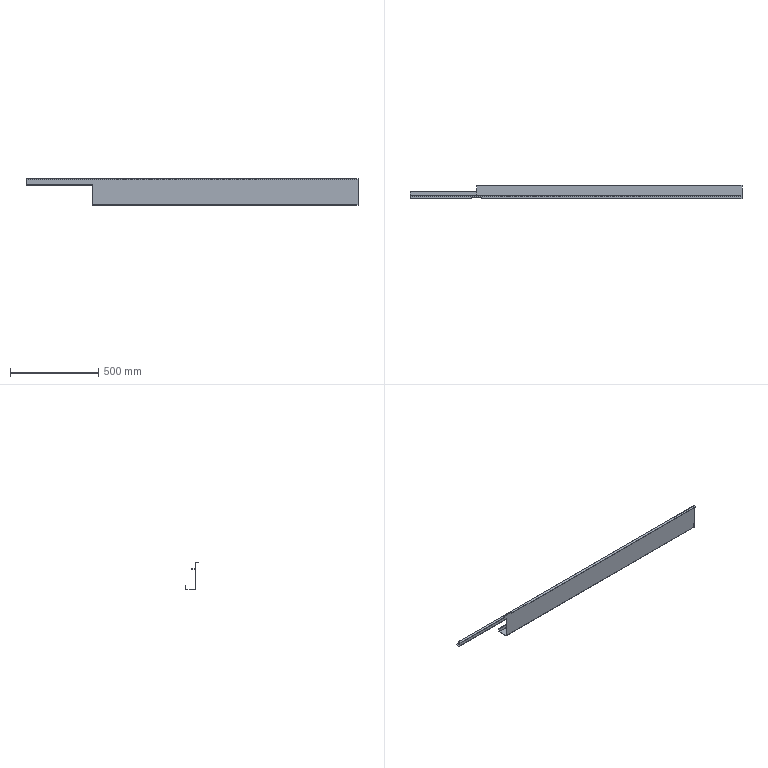Part | STEP file | Rear Base Frame | 1 solid | 32 faces | box 1881 x 75 x 152 mm | volume 779806 mm3 | plane 23 | cylinder 9 | commonest cylinder face diameters 1 x5 5 x4
STEP:
#1=CARTESIAN_POINT('',(1.,-1.349,2.843));
#2=VERTEX_POINT('',#1);
#3=CARTESIAN_POINT('',(1.,-1.349,6.343));
#4=VERTEX_POINT('',#3);
#5=CARTESIAN_POINT('',(1.,-1.349,37.843));
#6=DIRECTION('',(0.,0.,1.));
#7=VECTOR('',#6,1000.);
#8=LINE('',#5,#7);
#9=EDGE_CURVE('',#2,#4,#8,.T.);
#10=ORIENTED_EDGE('',*,*,#9,.T.);
#11=CARTESIAN_POINT('',(0.,-1.349,6.343));
#12=VERTEX_POINT('',#11);
#13=CARTESIAN_POINT('',(0.5,-1.349,6.343));
#14=DIRECTION('',(0.,-1.,0.));
#15=DIRECTION('',(0.,0.,-1.));
#16=AXIS2_PLACEMENT_3D('',#13,#14,#15);
#17=CIRCLE('',#16,0.5);
#18=EDGE_CURVE('',#4,#12,#17,.T.);
#19=ORIENTED_EDGE('',*,*,#18,.T.);
#20=CARTESIAN_POINT('',(0.,-1.349,5.343));
#21=VERTEX_POINT('',#20);
#22=CARTESIAN_POINT('',(0.,-1.349,5.343));
#23=DIRECTION('',(0.,0.,1.));
#24=VECTOR('',#23,1000.);
#25=LINE('',#22,#24);
#26=EDGE_CURVE('',#21,#12,#25,.T.);
#27=ORIENTED_EDGE('',*,*,#26,.F.);
#28=CARTESIAN_POINT('',(-377.,-1.349,5.343));
#29=VERTEX_POINT('',#28);
#30=CARTESIAN_POINT('',(1504.,-1.349,5.343));
#31=DIRECTION('',(-1.,0.,0.));
#32=VECTOR('',#31,1000.);
#33=LINE('',#30,#32);
#34=EDGE_CURVE('',#21,#29,#33,.T.);
#35=ORIENTED_EDGE('',*,*,#34,.T.);
#36=CARTESIAN_POINT('',(-377.,-1.349,37.343));
#37=VERTEX_POINT('',#36);
#38=CARTESIAN_POINT('',(-377.,-1.349,37.843));
#39=DIRECTION('',(0.,0.,1.));
#40=VECTOR('',#39,1000.);
#41=LINE('',#38,#40);
#42=EDGE_CURVE('',#29,#37,#41,.T.);
#43=ORIENTED_EDGE('',*,*,#42,.T.);
#44=CARTESIAN_POINT('',(1504.,-1.349,37.343));
#45=VERTEX_POINT('',#44);
#46=CARTESIAN_POINT('',(1504.,-1.349,37.343));
#47=DIRECTION('',(1.,0.,0.));
#48=VECTOR('',#47,1000.);
#49=LINE('',#46,#48);
#50=EDGE_CURVE('',#37,#45,#49,.T.);
#51=ORIENTED_EDGE('',*,*,#50,.T.);
#52=CARTESIAN_POINT('',(1504.,-1.349,-109.657));
#53=VERTEX_POINT('',#52);
#54=CARTESIAN_POINT('',(1504.,-1.349,37.843));
#55=DIRECTION('',(0.,0.,-1.));
#56=VECTOR('',#55,1000.);
#57=LINE('',#54,#56);
#58=EDGE_CURVE('',#45,#53,#57,.T.);
#59=ORIENTED_EDGE('',*,*,#58,.T.);
#60=CARTESIAN_POINT('',(0.,-1.349,-109.657));
#61=VERTEX_POINT('',#60);
#62=CARTESIAN_POINT('',(1504.,-1.349,-109.657));
#63=DIRECTION('',(-1.,0.,0.));
#64=VECTOR('',#63,1000.);
#65=LINE('',#62,#64);
#66=EDGE_CURVE('',#53,#61,#65,.T.);
#67=ORIENTED_EDGE('',*,*,#66,.T.);
#68=CARTESIAN_POINT('',(0.,-1.349,2.843));
#69=VERTEX_POINT('',#68);
#70=CARTESIAN_POINT('',(0.,-1.349,37.843));
#71=DIRECTION('',(0.,0.,1.));
#72=VECTOR('',#71,1000.);
#73=LINE('',#70,#72);
#74=EDGE_CURVE('',#61,#69,#73,.T.);
#75=ORIENTED_EDGE('',*,*,#74,.T.);
#76=CARTESIAN_POINT('',(1.,-1.349,2.843));
#77=DIRECTION('',(-1.,0.,0.));
#78=VECTOR('',#77,1000.);
#79=LINE('',#76,#78);
#80=EDGE_CURVE('',#2,#69,#79,.T.);
#81=ORIENTED_EDGE('',*,*,#80,.F.);
#82=EDGE_LOOP('',(#10,#19,#27,#35,#43,#51,#59,#67,#75,#81));
#83=FACE_OUTER_BOUND('',#82,.T.);
#84=CARTESIAN_POINT('',(1504.,-1.349,37.843));
#85=DIRECTION('',(0.,1.,0.));
#86=DIRECTION('',(0.,0.,1.));
#87=AXIS2_PLACEMENT_3D('',#84,#85,#86);
#88=PLANE('',#87);
#89=ADVANCED_FACE('',(#83),#88,.T.);
#90=CARTESIAN_POINT('',(1.,-3.349,6.343));
#91=VERTEX_POINT('',#90);
#92=CARTESIAN_POINT('',(1.,-1.349,6.343));
#93=DIRECTION('',(0.,1.,0.));
#94=VECTOR('',#93,1000.);
#95=LINE('',#92,#94);
#96=EDGE_CURVE('',#91,#4,#95,.T.);
#97=ORIENTED_EDGE('',*,*,#96,.T.);
#98=ORIENTED_EDGE('',*,*,#9,.F.);
#99=CARTESIAN_POINT('',(1.,-3.349,2.843));
#100=VERTEX_POINT('',#99);
#101=CARTESIAN_POINT('',(1.,-1.349,2.843));
#102=DIRECTION('',(0.,-1.,0.));
#103=VECTOR('',#102,1000.);
#104=LINE('',#101,#103);
#105=EDGE_CURVE('',#2,#100,#104,.T.);
#106=ORIENTED_EDGE('',*,*,#105,.T.);
#107=CARTESIAN_POINT('',(1.,-3.349,6.343));
#108=DIRECTION('',(0.,0.,1.));
#109=VECTOR('',#108,1000.);
#110=LINE('',#107,#109);
#111=EDGE_CURVE('',#100,#91,#110,.T.);
#112=ORIENTED_EDGE('',*,*,#111,.T.);
#113=EDGE_LOOP('',(#97,#98,#106,#112));
#114=FACE_OUTER_BOUND('',#113,.T.);
#115=CARTESIAN_POINT('',(1.,-1.349,6.343));
#116=DIRECTION('',(-1.,0.,0.));
#117=DIRECTION('',(0.,0.,1.));
#118=AXIS2_PLACEMENT_3D('',#115,#116,#117);
#119=PLANE('',#118);
#120=ADVANCED_FACE('',(#114),#119,.T.);
#121=ORIENTED_EDGE('',*,*,#74,.F.);
#122=CARTESIAN_POINT('',(0.,-0.8487,-110.157));
#123=VERTEX_POINT('',#122);
#124=CARTESIAN_POINT('',(0.,-0.8487,-109.657));
#125=DIRECTION('',(1.,0.,0.));
#126=DIRECTION('',(0.,0.,1.));
#127=AXIS2_PLACEMENT_3D('',#124,#125,#126);
#128=CIRCLE('',#127,0.5);
#129=EDGE_CURVE('',#61,#123,#128,.T.);
#130=ORIENTED_EDGE('',*,*,#129,.T.);
#131=CARTESIAN_POINT('',(0.,54.151,-110.157));
#132=VERTEX_POINT('',#131);
#133=CARTESIAN_POINT('',(0.,-3.349,-110.157));
#134=DIRECTION('',(0.,-1.,0.));
#135=VECTOR('',#134,1000.);
#136=LINE('',#133,#135);
#137=EDGE_CURVE('',#132,#123,#136,.T.);
#138=ORIENTED_EDGE('',*,*,#137,.F.);
#139=CARTESIAN_POINT('',(0.,54.651,-109.657));
#140=VERTEX_POINT('',#139);
#141=CARTESIAN_POINT('',(0.,54.151,-109.657));
#142=DIRECTION('',(1.,0.,0.));
#143=DIRECTION('',(0.,0.,1.));
#144=AXIS2_PLACEMENT_3D('',#141,#142,#143);
#145=CIRCLE('',#144,0.5);
#146=EDGE_CURVE('',#132,#140,#145,.T.);
#147=ORIENTED_EDGE('',*,*,#146,.T.);
#148=CARTESIAN_POINT('',(0.,54.651,-92.157));
#149=VERTEX_POINT('',#148);
#150=CARTESIAN_POINT('',(0.,54.651,-112.157));
#151=DIRECTION('',(0.,0.,-1.));
#152=VECTOR('',#151,1000.);
#153=LINE('',#150,#152);
#154=EDGE_CURVE('',#149,#140,#153,.T.);
#155=ORIENTED_EDGE('',*,*,#154,.F.);
#156=CARTESIAN_POINT('',(0.,56.651,-92.157));
#157=VERTEX_POINT('',#156);
#158=CARTESIAN_POINT('',(0.,54.151,-92.157));
#159=DIRECTION('',(0.,1.,0.));
#160=VECTOR('',#159,1000.);
#161=LINE('',#158,#160);
#162=EDGE_CURVE('',#149,#157,#161,.T.);
#163=ORIENTED_EDGE('',*,*,#162,.T.);
#164=CARTESIAN_POINT('',(0.,56.651,-109.657));
#165=VERTEX_POINT('',#164);
#166=CARTESIAN_POINT('',(0.,56.651,-110.157));
#167=DIRECTION('',(0.,0.,-1.));
#168=VECTOR('',#167,1000.);
#169=LINE('',#166,#168);
#170=EDGE_CURVE('',#157,#165,#169,.T.);
#171=ORIENTED_EDGE('',*,*,#170,.T.);
#172=CARTESIAN_POINT('',(0.,54.151,-112.157));
#173=VERTEX_POINT('',#172);
#174=CARTESIAN_POINT('',(0.,54.151,-109.657));
#175=DIRECTION('',(-1.,0.,0.));
#176=DIRECTION('',(0.,0.,1.));
#177=AXIS2_PLACEMENT_3D('',#174,#175,#176);
#178=CIRCLE('',#177,2.5);
#179=EDGE_CURVE('',#165,#173,#178,.T.);
#180=ORIENTED_EDGE('',*,*,#179,.T.);
#181=CARTESIAN_POINT('',(0.,-0.8487,-112.157));
#182=VERTEX_POINT('',#181);
#183=CARTESIAN_POINT('',(0.,-1.349,-112.157));
#184=DIRECTION('',(0.,-1.,0.));
#185=VECTOR('',#184,1000.);
#186=LINE('',#183,#185);
#187=EDGE_CURVE('',#173,#182,#186,.T.);
#188=ORIENTED_EDGE('',*,*,#187,.T.);
#189=CARTESIAN_POINT('',(0.,-3.349,-109.657));
#190=VERTEX_POINT('',#189);
#191=CARTESIAN_POINT('',(0.,-0.8487,-109.657));
#192=DIRECTION('',(-1.,0.,0.));
#193=DIRECTION('',(0.,0.,1.));
#194=AXIS2_PLACEMENT_3D('',#191,#192,#193);
#195=CIRCLE('',#194,2.5);
#196=EDGE_CURVE('',#182,#190,#195,.T.);
#197=ORIENTED_EDGE('',*,*,#196,.T.);
#198=CARTESIAN_POINT('',(0.,-3.349,2.843));
#199=VERTEX_POINT('',#198);
#200=CARTESIAN_POINT('',(0.,-3.349,39.843));
#201=DIRECTION('',(0.,0.,1.));
#202=VECTOR('',#201,1000.);
#203=LINE('',#200,#202);
#204=EDGE_CURVE('',#190,#199,#203,.T.);
#205=ORIENTED_EDGE('',*,*,#204,.T.);
#206=CARTESIAN_POINT('',(0.,-3.849,2.843));
#207=DIRECTION('',(0.,1.,0.));
#208=VECTOR('',#207,1000.);
#209=LINE('',#206,#208);
#210=EDGE_CURVE('',#199,#69,#209,.T.);
#211=ORIENTED_EDGE('',*,*,#210,.T.);
#212=EDGE_LOOP('',(#121,#130,#138,#147,#155,#163,#171,#180,#188,#197,#205,#211));
#213=FACE_OUTER_BOUND('',#212,.T.);
#214=CARTESIAN_POINT('',(0.,-3.849,39.843));
#215=DIRECTION('',(-1.,0.,0.));
#216=DIRECTION('',(0.,0.,1.));
#217=AXIS2_PLACEMENT_3D('',#214,#215,#216);
#218=PLANE('',#217);
#219=ADVANCED_FACE('',(#213),#218,.T.);
#220=ORIENTED_EDGE('',*,*,#66,.F.);
#221=CARTESIAN_POINT('',(1504.,-0.8487,-110.157));
#222=VERTEX_POINT('',#221);
#223=CARTESIAN_POINT('',(1504.,-0.8487,-109.657));
#224=DIRECTION('',(-1.,0.,0.));
#225=DIRECTION('',(0.,0.,1.));
#226=AXIS2_PLACEMENT_3D('',#223,#224,#225);
#227=CIRCLE('',#226,0.5);
#228=EDGE_CURVE('',#222,#53,#227,.T.);
#229=ORIENTED_EDGE('',*,*,#228,.F.);
#230=CARTESIAN_POINT('',(1504.,-0.8487,-110.157));
#231=DIRECTION('',(1.,0.,0.));
#232=VECTOR('',#231,1000.);
#233=LINE('',#230,#232);
#234=EDGE_CURVE('',#123,#222,#233,.T.);
#235=ORIENTED_EDGE('',*,*,#234,.F.);
#236=ORIENTED_EDGE('',*,*,#129,.F.);
#237=EDGE_LOOP('',(#220,#229,#235,#236));
#238=FACE_OUTER_BOUND('',#237,.T.);
#239=CARTESIAN_POINT('',(1504.,-0.8487,-109.657));
#240=DIRECTION('',(-1.,0.,0.));
#241=DIRECTION('',(0.,0.,1.));
#242=AXIS2_PLACEMENT_3D('',#239,#240,#241);
#243=CYLINDRICAL_SURFACE('',#242,0.5);
#244=ADVANCED_FACE('',(#238),#243,.F.);
#245=ORIENTED_EDGE('',*,*,#58,.F.);
#246=CARTESIAN_POINT('',(1504.,-3.849,39.843));
#247=VERTEX_POINT('',#246);
#248=CARTESIAN_POINT('',(1504.,-3.849,37.343));
#249=DIRECTION('',(-1.,0.,0.));
#250=DIRECTION('',(0.,0.,1.));
#251=AXIS2_PLACEMENT_3D('',#248,#249,#250);
#252=CIRCLE('',#251,2.5);
#253=EDGE_CURVE('',#247,#45,#252,.T.);
#254=ORIENTED_EDGE('',*,*,#253,.F.);
#255=CARTESIAN_POINT('',(1504.,-18.349,39.843));
#256=VERTEX_POINT('',#255);
#257=CARTESIAN_POINT('',(1504.,-18.349,39.843));
#258=DIRECTION('',(0.,1.,0.));
#259=VECTOR('',#258,1000.);
#260=LINE('',#257,#259);
#261=EDGE_CURVE('',#256,#247,#260,.T.);
#262=ORIENTED_EDGE('',*,*,#261,.F.);
#263=CARTESIAN_POINT('',(1504.,-18.349,37.843));
#264=VERTEX_POINT('',#263);
#265=CARTESIAN_POINT('',(1504.,-18.349,37.343));
#266=DIRECTION('',(0.,0.,-1.));
#267=VECTOR('',#266,1000.);
#268=LINE('',#265,#267);
#269=EDGE_CURVE('',#256,#264,#268,.T.);
#270=ORIENTED_EDGE('',*,*,#269,.T.);
#271=CARTESIAN_POINT('',(1504.,-3.849,37.843));
#272=VERTEX_POINT('',#271);
#273=CARTESIAN_POINT('',(1504.,-18.349,37.843));
#274=DIRECTION('',(0.,1.,0.));
#275=VECTOR('',#274,1000.);
#276=LINE('',#273,#275);
#277=EDGE_CURVE('',#264,#272,#276,.T.);
#278=ORIENTED_EDGE('',*,*,#277,.T.);
#279=CARTESIAN_POINT('',(1504.,-3.349,37.343));
#280=VERTEX_POINT('',#279);
#281=CARTESIAN_POINT('',(1504.,-3.849,37.343));
#282=DIRECTION('',(-1.,0.,0.));
#283=DIRECTION('',(0.,0.,1.));
#284=AXIS2_PLACEMENT_3D('',#281,#282,#283);
#285=CIRCLE('',#284,0.5);
#286=EDGE_CURVE('',#272,#280,#285,.T.);
#287=ORIENTED_EDGE('',*,*,#286,.T.);
#288=CARTESIAN_POINT('',(1504.,-3.349,-109.657));
#289=VERTEX_POINT('',#288);
#290=CARTESIAN_POINT('',(1504.,-3.349,-110.157));
#291=DIRECTION('',(0.,0.,-1.));
#292=VECTOR('',#291,1000.);
#293=LINE('',#290,#292);
#294=EDGE_CURVE('',#280,#289,#293,.T.);
#295=ORIENTED_EDGE('',*,*,#294,.T.);
#296=CARTESIAN_POINT('',(1504.,-0.8487,-112.157));
#297=VERTEX_POINT('',#296);
#298=CARTESIAN_POINT('',(1504.,-0.8487,-109.657));
#299=DIRECTION('',(1.,0.,0.));
#300=DIRECTION('',(0.,0.,1.));
#301=AXIS2_PLACEMENT_3D('',#298,#299,#300);
#302=CIRCLE('',#301,2.5);
#303=EDGE_CURVE('',#289,#297,#302,.T.);
#304=ORIENTED_EDGE('',*,*,#303,.T.);
#305=CARTESIAN_POINT('',(1504.,54.151,-112.157));
#306=VERTEX_POINT('',#305);
#307=CARTESIAN_POINT('',(1504.,54.651,-112.157));
#308=DIRECTION('',(0.,1.,0.));
#309=VECTOR('',#308,1000.);
#310=LINE('',#307,#309);
#311=EDGE_CURVE('',#297,#306,#310,.T.);
#312=ORIENTED_EDGE('',*,*,#311,.T.);
#313=CARTESIAN_POINT('',(1504.,56.651,-109.657));
#314=VERTEX_POINT('',#313);
#315=CARTESIAN_POINT('',(1504.,54.151,-109.657));
#316=DIRECTION('',(1.,0.,0.));
#317=DIRECTION('',(0.,0.,1.));
#318=AXIS2_PLACEMENT_3D('',#315,#316,#317);
#319=CIRCLE('',#318,2.5);
#320=EDGE_CURVE('',#306,#314,#319,.T.);
#321=ORIENTED_EDGE('',*,*,#320,.T.);
#322=CARTESIAN_POINT('',(1504.,56.651,-92.157));
#323=VERTEX_POINT('',#322);
#324=CARTESIAN_POINT('',(1504.,56.651,-109.657));
#325=DIRECTION('',(0.,0.,1.));
#326=VECTOR('',#325,1000.);
#327=LINE('',#324,#326);
#328=EDGE_CURVE('',#314,#323,#327,.T.);
#329=ORIENTED_EDGE('',*,*,#328,.T.);
#330=CARTESIAN_POINT('',(1504.,54.651,-92.157));
#331=VERTEX_POINT('',#330);
#332=CARTESIAN_POINT('',(1504.,54.651,-92.157));
#333=DIRECTION('',(0.,1.,0.));
#334=VECTOR('',#333,1000.);
#335=LINE('',#332,#334);
#336=EDGE_CURVE('',#331,#323,#335,.T.);
#337=ORIENTED_EDGE('',*,*,#336,.F.);
#338=CARTESIAN_POINT('',(1504.,54.651,-109.657));
#339=VERTEX_POINT('',#338);
#340=CARTESIAN_POINT('',(1504.,54.651,-112.157));
#341=DIRECTION('',(0.,0.,1.));
#342=VECTOR('',#341,1000.);
#343=LINE('',#340,#342);
#344=EDGE_CURVE('',#339,#331,#343,.T.);
#345=ORIENTED_EDGE('',*,*,#344,.F.);
#346=CARTESIAN_POINT('',(1504.,54.151,-110.157));
#347=VERTEX_POINT('',#346);
#348=CARTESIAN_POINT('',(1504.,54.151,-109.657));
#349=DIRECTION('',(-1.,0.,0.));
#350=DIRECTION('',(0.,0.,1.));
#351=AXIS2_PLACEMENT_3D('',#348,#349,#350);
#352=CIRCLE('',#351,0.5);
#353=EDGE_CURVE('',#339,#347,#352,.T.);
#354=ORIENTED_EDGE('',*,*,#353,.T.);
#355=CARTESIAN_POINT('',(1504.,-3.349,-110.157));
#356=DIRECTION('',(0.,1.,0.));
#357=VECTOR('',#356,1000.);
#358=LINE('',#355,#357);
#359=EDGE_CURVE('',#222,#347,#358,.T.);
#360=ORIENTED_EDGE('',*,*,#359,.F.);
#361=ORIENTED_EDGE('',*,*,#228,.T.);
#362=EDGE_LOOP('',(#245,#254,#262,#270,#278,#287,#295,#304,#312,#321,#329,#337,#345,#354,#360,#361));
#363=FACE_OUTER_BOUND('',#362,.T.);
#364=CARTESIAN_POINT('',(1504.,-0.8487,-110.157));
#365=DIRECTION('',(1.,0.,0.));
#366=DIRECTION('',(0.,0.,-1.));
#367=AXIS2_PLACEMENT_3D('',#364,#365,#366);
#368=PLANE('',#367);
#369=ADVANCED_FACE('',(#363),#368,.T.);
#370=CARTESIAN_POINT('',(-377.,-3.849,39.843));
#371=VERTEX_POINT('',#370);
#372=CARTESIAN_POINT('',(1504.,-3.849,39.843));
#373=DIRECTION('',(1.,0.,0.));
#374=VECTOR('',#373,1000.);
#375=LINE('',#372,#374);
#376=EDGE_CURVE('',#371,#247,#375,.T.);
#377=ORIENTED_EDGE('',*,*,#376,.T.);
#378=ORIENTED_EDGE('',*,*,#253,.T.);
#379=ORIENTED_EDGE('',*,*,#50,.F.);
#380=CARTESIAN_POINT('',(-377.,-3.849,37.343));
#381=DIRECTION('',(1.,0.,0.));
#382=DIRECTION('',(0.,0.,1.));
#383=AXIS2_PLACEMENT_3D('',#380,#381,#382);
#384=CIRCLE('',#383,2.5);
#385=EDGE_CURVE('',#37,#371,#384,.T.);
#386=ORIENTED_EDGE('',*,*,#385,.T.);
#387=EDGE_LOOP('',(#377,#378,#379,#386));
#388=FACE_OUTER_BOUND('',#387,.T.);
#389=CARTESIAN_POINT('',(1504.,-3.849,37.343));
#390=DIRECTION('',(-1.,0.,0.));
#391=DIRECTION('',(0.,0.,1.));
#392=AXIS2_PLACEMENT_3D('',#389,#390,#391);
#393=CYLINDRICAL_SURFACE('',#392,2.5);
#394=ADVANCED_FACE('',(#388),#393,.T.);
#395=CARTESIAN_POINT('',(-377.,-18.349,39.843));
#396=VERTEX_POINT('',#395);
#397=CARTESIAN_POINT('',(-377.,-3.849,39.843));
#398=DIRECTION('',(0.,1.,0.));
#399=VECTOR('',#398,1000.);
#400=LINE('',#397,#399);
#401=EDGE_CURVE('',#396,#371,#400,.T.);
#402=ORIENTED_EDGE('',*,*,#401,.T.);
#403=ORIENTED_EDGE('',*,*,#385,.F.);
#404=ORIENTED_EDGE('',*,*,#42,.F.);
#405=CARTESIAN_POINT('',(-377.,-0.8487,4.843));
#406=VERTEX_POINT('',#405);
#407=CARTESIAN_POINT('',(-377.,-0.8487,5.343));
#408=DIRECTION('',(1.,0.,0.));
#409=DIRECTION('',(0.,0.,1.));
#410=AXIS2_PLACEMENT_3D('',#407,#408,#409);
#411=CIRCLE('',#410,0.5);
#412=EDGE_CURVE('',#29,#406,#411,.T.);
#413=ORIENTED_EDGE('',*,*,#412,.T.);
#414=CARTESIAN_POINT('',(-377.,21.651,4.843));
#415=VERTEX_POINT('',#414);
#416=CARTESIAN_POINT('',(-377.,0.,4.843));
#417=DIRECTION('',(0.,1.,0.));
#418=VECTOR('',#417,1000.);
#419=LINE('',#416,#418);
#420=EDGE_CURVE('',#406,#415,#419,.T.);
#421=ORIENTED_EDGE('',*,*,#420,.T.);
#422=CARTESIAN_POINT('',(-377.,21.651,2.843));
#423=VERTEX_POINT('',#422);
#424=CARTESIAN_POINT('',(-377.,21.651,2.843));
#425=DIRECTION('',(0.,0.,-1.));
#426=VECTOR('',#425,1000.);
#427=LINE('',#424,#426);
#428=EDGE_CURVE('',#415,#423,#427,.T.);
#429=ORIENTED_EDGE('',*,*,#428,.T.);
#430=CARTESIAN_POINT('',(-377.,-0.8487,2.843));
#431=VERTEX_POINT('',#430);
#432=CARTESIAN_POINT('',(-377.,-1.349,2.843));
#433=DIRECTION('',(0.,-1.,0.));
#434=VECTOR('',#433,1000.);
#435=LINE('',#432,#434);
#436=EDGE_CURVE('',#423,#431,#435,.T.);
#437=ORIENTED_EDGE('',*,*,#436,.T.);
#438=CARTESIAN_POINT('',(-377.,-3.349,5.343));
#439=VERTEX_POINT('',#438);
#440=CARTESIAN_POINT('',(-377.,-0.8487,5.343));
#441=DIRECTION('',(1.,0.,0.));
#442=DIRECTION('',(0.,0.,1.));
#443=AXIS2_PLACEMENT_3D('',#440,#441,#442);
#444=CIRCLE('',#443,2.5);
#445=EDGE_CURVE('',#439,#431,#444,.T.);
#446=ORIENTED_EDGE('',*,*,#445,.F.);
#447=CARTESIAN_POINT('',(-377.,-3.349,37.343));
#448=VERTEX_POINT('',#447);
#449=CARTESIAN_POINT('',(-377.,-3.349,37.343));
#450=DIRECTION('',(0.,0.,1.));
#451=VECTOR('',#450,1000.);
#452=LINE('',#449,#451);
#453=EDGE_CURVE('',#439,#448,#452,.T.);
#454=ORIENTED_EDGE('',*,*,#453,.T.);
#455=CARTESIAN_POINT('',(-377.,-3.849,37.843));
#456=VERTEX_POINT('',#455);
#457=CARTESIAN_POINT('',(-377.,-3.849,37.343));
#458=DIRECTION('',(1.,0.,0.));
#459=DIRECTION('',(0.,0.,1.));
#460=AXIS2_PLACEMENT_3D('',#457,#458,#459);
#461=CIRCLE('',#460,0.5);
#462=EDGE_CURVE('',#448,#456,#461,.T.);
#463=ORIENTED_EDGE('',*,*,#462,.T.);
#464=CARTESIAN_POINT('',(-377.,-18.349,37.843));
#465=VERTEX_POINT('',#464);
#466=CARTESIAN_POINT('',(-377.,-3.849,37.843));
#467=DIRECTION('',(0.,-1.,0.));
#468=VECTOR('',#467,1000.);
#469=LINE('',#466,#468);
#470=EDGE_CURVE('',#456,#465,#469,.T.);
#471=ORIENTED_EDGE('',*,*,#470,.T.);
#472=CARTESIAN_POINT('',(-377.,-18.349,37.343));
#473=DIRECTION('',(0.,0.,1.));
#474=VECTOR('',#473,1000.);
#475=LINE('',#472,#474);
#476=EDGE_CURVE('',#465,#396,#475,.T.);
#477=ORIENTED_EDGE('',*,*,#476,.T.);
#478=EDGE_LOOP('',(#402,#403,#404,#413,#421,#429,#437,#446,#454,#463,#471,#477));
#479=FACE_OUTER_BOUND('',#478,.T.);
#480=CARTESIAN_POINT('',(-377.,-3.849,37.343));
#481=DIRECTION('',(-1.,0.,0.));
#482=DIRECTION('',(0.,0.,1.));
#483=AXIS2_PLACEMENT_3D('',#480,#481,#482);
#484=PLANE('',#483);
#485=ADVANCED_FACE('',(#479),#484,.T.);
#486=CARTESIAN_POINT('',(0.,-0.8487,4.843));
#487=VERTEX_POINT('',#486);
#488=CARTESIAN_POINT('',(0.,-0.8487,5.343));
#489=DIRECTION('',(-1.,0.,0.));
#490=DIRECTION('',(0.,0.,1.));
#491=AXIS2_PLACEMENT_3D('',#488,#489,#490);
#492=CIRCLE('',#491,0.5);
#493=EDGE_CURVE('',#487,#21,#492,.T.);
#494=ORIENTED_EDGE('',*,*,#493,.F.);
#495=CARTESIAN_POINT('',(-377.,-0.8487,4.843));
#496=DIRECTION('',(1.,0.,0.));
#497=VECTOR('',#496,1000.);
#498=LINE('',#495,#497);
#499=EDGE_CURVE('',#406,#487,#498,.T.);
#500=ORIENTED_EDGE('',*,*,#499,.F.);
#501=ORIENTED_EDGE('',*,*,#412,.F.);
#502=ORIENTED_EDGE('',*,*,#34,.F.);
#503=EDGE_LOOP('',(#494,#500,#501,#502));
#504=FACE_OUTER_BOUND('',#503,.T.);
#505=CARTESIAN_POINT('',(-377.,-0.8487,5.343));
#506=DIRECTION('',(-1.,0.,0.));
#507=DIRECTION('',(0.,0.,1.));
#508=AXIS2_PLACEMENT_3D('',#505,#506,#507);
#509=CYLINDRICAL_SURFACE('',#508,0.5);
#510=ADVANCED_FACE('',(#504),#509,.F.);
#511=CARTESIAN_POINT('',(0.,-3.349,6.343));
#512=VERTEX_POINT('',#511);
#513=CARTESIAN_POINT('',(0.5,-3.349,6.343));
#514=DIRECTION('',(0.,1.,0.));
#515=DIRECTION('',(0.,0.,-1.));
#516=AXIS2_PLACEMENT_3D('',#513,#514,#515);
#517=CIRCLE('',#516,0.5);
#518=EDGE_CURVE('',#512,#91,#517,.T.);
#519=ORIENTED_EDGE('',*,*,#518,.F.);
#520=CARTESIAN_POINT('',(0.,-1.349,6.343));
#521=DIRECTION('',(0.,-1.,0.));
#522=VECTOR('',#521,1000.);
#523=LINE('',#520,#522);
#524=EDGE_CURVE('',#12,#512,#523,.T.);
#525=ORIENTED_EDGE('',*,*,#524,.F.);
#526=ORIENTED_EDGE('',*,*,#18,.F.);
#527=ORIENTED_EDGE('',*,*,#96,.F.);
#528=EDGE_LOOP('',(#519,#525,#526,#527));
#529=FACE_OUTER_BOUND('',#528,.T.);
#530=CARTESIAN_POINT('',(0.5,-1.349,6.343));
#531=DIRECTION('',(0.,-1.,0.));
#532=DIRECTION('',(0.,0.,-1.));
#533=AXIS2_PLACEMENT_3D('',#530,#531,#532);
#534=CYLINDRICAL_SURFACE('',#533,0.5);
#535=ADVANCED_FACE('',(#529),#534,.F.);
#536=CARTESIAN_POINT('',(0.,-3.349,5.343));
#537=VERTEX_POINT('',#536);
#538=CARTESIAN_POINT('',(0.,-3.349,37.843));
#539=DIRECTION('',(0.,0.,-1.));
#540=VECTOR('',#539,1000.);
#541=LINE('',#538,#540);
#542=EDGE_CURVE('',#512,#537,#541,.T.);
#543=ORIENTED_EDGE('',*,*,#542,.F.);
#544=ORIENTED_EDGE('',*,*,#518,.T.);
#545=ORIENTED_EDGE('',*,*,#111,.F.);
#546=CARTESIAN_POINT('',(1504.,-3.349,2.843));
#547=DIRECTION('',(1.,0.,0.));
#548=VECTOR('',#547,1000.);
#549=LINE('',#546,#548);
#550=EDGE_CURVE('',#199,#100,#549,.T.);
#551=ORIENTED_EDGE('',*,*,#550,.F.);
#552=ORIENTED_EDGE('',*,*,#204,.F.);
#553=CARTESIAN_POINT('',(1504.,-3.349,-109.657));
#554=DIRECTION('',(-1.,0.,0.));
#555=VECTOR('',#554,1000.);
#556=LINE('',#553,#555);
#557=EDGE_CURVE('',#289,#190,#556,.T.);
#558=ORIENTED_EDGE('',*,*,#557,.F.);
#559=ORIENTED_EDGE('',*,*,#294,.F.);
#560=CARTESIAN_POINT('',(1504.,-3.349,37.343));
#561=DIRECTION('',(1.,0.,0.));
#562=VECTOR('',#561,1000.);
#563=LINE('',#560,#562);
#564=EDGE_CURVE('',#448,#280,#563,.T.);
#565=ORIENTED_EDGE('',*,*,#564,.F.);
#566=ORIENTED_EDGE('',*,*,#453,.F.);
#567=CARTESIAN_POINT('',(1504.,-3.349,5.343));
#568=DIRECTION('',(-1.,0.,0.));
#569=VECTOR('',#568,1000.);
#570=LINE('',#567,#569);
#571=EDGE_CURVE('',#537,#439,#570,.T.);
#572=ORIENTED_EDGE('',*,*,#571,.F.);
#573=EDGE_LOOP('',(#543,#544,#545,#551,#552,#558,#559,#565,#566,#572));
#574=FACE_OUTER_BOUND('',#573,.T.);
#575=CARTESIAN_POINT('',(1504.,-3.349,37.843));
#576=DIRECTION('',(0.,1.,0.));
#577=DIRECTION('',(0.,0.,1.));
#578=AXIS2_PLACEMENT_3D('',#575,#576,#577);
#579=PLANE('',#578);
#580=ADVANCED_FACE('',(#574),#579,.F.);
#581=ORIENTED_EDGE('',*,*,#105,.F.);
#582=ORIENTED_EDGE('',*,*,#80,.T.);
#583=ORIENTED_EDGE('',*,*,#210,.F.);
#584=ORIENTED_EDGE('',*,*,#550,.T.);
#585=EDGE_LOOP('',(#581,#582,#583,#584));
#586=FACE_OUTER_BOUND('',#585,.T.);
#587=CARTESIAN_POINT('',(1.,-1.349,2.843));
#588=DIRECTION('',(0.,0.,1.));
#589=DIRECTION('',(0.,-1.,0.));
#590=AXIS2_PLACEMENT_3D('',#587,#588,#589);
#591=PLANE('',#590);
#592=ADVANCED_FACE('',(#586),#591,.T.);
#593=ORIENTED_EDGE('',*,*,#359,.T.);
#594=CARTESIAN_POINT('',(1504.,54.151,-110.157));
#595=DIRECTION('',(-1.,0.,0.));
#596=VECTOR('',#595,1000.);
#597=LINE('',#594,#596);
#598=EDGE_CURVE('',#347,#132,#597,.T.);
#599=ORIENTED_EDGE('',*,*,#598,.T.);
#600=ORIENTED_EDGE('',*,*,#137,.T.);
#601=ORIENTED_EDGE('',*,*,#234,.T.);
#602=EDGE_LOOP('',(#593,#599,#600,#601));
#603=FACE_OUTER_BOUND('',#602,.T.);
#604=CARTESIAN_POINT('',(1504.,-3.349,-110.157));
#605=DIRECTION('',(0.,0.,1.));
#606=DIRECTION('',(1.,0.,0.));
#607=AXIS2_PLACEMENT_3D('',#604,#605,#606);
#608=PLANE('',#607);
#609=ADVANCED_FACE('',(#603),#608,.T.);
#610=ORIENTED_EDGE('',*,*,#401,.F.);
#611=CARTESIAN_POINT('',(-30.,-18.349,39.843));
#612=VERTEX_POINT('',#611);
#613=CARTESIAN_POINT('',(1504.,-18.349,39.843));
#614=DIRECTION('',(1.,0.,0.));
#615=VECTOR('',#614,1000.);
#616=LINE('',#613,#615);
#617=EDGE_CURVE('',#396,#612,#616,.T.);
#618=ORIENTED_EDGE('',*,*,#617,.T.);
#619=CARTESIAN_POINT('',(-30.,-10.849,39.843));
#620=VERTEX_POINT('',#619);
#621=CARTESIAN_POINT('',(-30.,-18.349,39.843));
#622=DIRECTION('',(0.,1.,0.));
#623=VECTOR('',#622,1000.);
#624=LINE('',#621,#623);
#625=EDGE_CURVE('',#612,#620,#624,.T.);
#626=ORIENTED_EDGE('',*,*,#625,.T.);
#627=CARTESIAN_POINT('',(30.,-10.849,39.843));
#628=VERTEX_POINT('',#627);
#629=CARTESIAN_POINT('',(1504.,-10.849,39.843));
#630=DIRECTION('',(1.,0.,0.));
#631=VECTOR('',#630,1000.);
#632=LINE('',#629,#631);
#633=EDGE_CURVE('',#620,#628,#632,.T.);
#634=ORIENTED_EDGE('',*,*,#633,.T.);
#635=CARTESIAN_POINT('',(30.,-18.349,39.843));
#636=VERTEX_POINT('',#635);
#637=CARTESIAN_POINT('',(30.,-18.349,39.843));
#638=DIRECTION('',(0.,-1.,0.));
#639=VECTOR('',#638,1000.);
#640=LINE('',#637,#639);
#641=EDGE_CURVE('',#628,#636,#640,.T.);
#642=ORIENTED_EDGE('',*,*,#641,.T.);
#643=CARTESIAN_POINT('',(1504.,-18.349,39.843));
#644=DIRECTION('',(1.,0.,0.));
#645=VECTOR('',#644,1000.);
#646=LINE('',#643,#645);
#647=EDGE_CURVE('',#636,#256,#646,.T.);
#648=ORIENTED_EDGE('',*,*,#647,.T.);
#649=ORIENTED_EDGE('',*,*,#261,.T.);
#650=ORIENTED_EDGE('',*,*,#376,.F.);
#651=EDGE_LOOP('',(#610,#618,#626,#634,#642,#648,#649,#650));
#652=FACE_OUTER_BOUND('',#651,.T.);
#653=CARTESIAN_POINT('',(1504.,-18.349,39.843));
#654=DIRECTION('',(0.,0.,1.));
#655=DIRECTION('',(1.,0.,0.));
#656=AXIS2_PLACEMENT_3D('',#653,#654,#655);
#657=PLANE('',#656);
#658=ADVANCED_FACE('',(#652),#657,.T.);
#659=ORIENTED_EDGE('',*,*,#476,.F.);
#660=CARTESIAN_POINT('',(-30.,-18.349,37.843));
#661=VERTEX_POINT('',#660);
#662=CARTESIAN_POINT('',(1504.,-18.349,37.843));
#663=DIRECTION('',(1.,0.,0.));
#664=VECTOR('',#663,1000.);
#665=LINE('',#662,#664);
#666=EDGE_CURVE('',#465,#661,#665,.T.);
#667=ORIENTED_EDGE('',*,*,#666,.T.);
#668=CARTESIAN_POINT('',(-30.,-18.349,37.843));
#669=DIRECTION('',(0.,0.,1.));
#670=VECTOR('',#669,1000.);
#671=LINE('',#668,#670);
#672=EDGE_CURVE('',#661,#612,#671,.T.);
#673=ORIENTED_EDGE('',*,*,#672,.T.);
#674=ORIENTED_EDGE('',*,*,#617,.F.);
#675=EDGE_LOOP('',(#659,#667,#673,#674));
#676=FACE_OUTER_BOUND('',#675,.T.);
#677=CARTESIAN_POINT('',(1504.,-18.349,37.843));
#678=DIRECTION('',(0.,-1.,0.));
#679=DIRECTION('',(0.,0.,-1.));
#680=AXIS2_PLACEMENT_3D('',#677,#678,#679);
#681=PLANE('',#680);
#682=ADVANCED_FACE('',(#676),#681,.T.);
#683=CARTESIAN_POINT('',(-30.,-10.849,37.843));
#684=VERTEX_POINT('',#683);
#685=CARTESIAN_POINT('',(-30.,-18.349,37.843));
#686=DIRECTION('',(0.,1.,0.));
#687=VECTOR('',#686,1000.);
#688=LINE('',#685,#687);
#689=EDGE_CURVE('',#661,#684,#688,.T.);
#690=ORIENTED_EDGE('',*,*,#689,.F.);
#691=ORIENTED_EDGE('',*,*,#666,.F.);
#692=ORIENTED_EDGE('',*,*,#470,.F.);
#693=CARTESIAN_POINT('',(1504.,-3.849,37.843));
#694=DIRECTION('',(-1.,0.,0.));
#695=VECTOR('',#694,1000.);
#696=LINE('',#693,#695);
#697=EDGE_CURVE('',#272,#456,#696,.T.);
#698=ORIENTED_EDGE('',*,*,#697,.F.);
#699=ORIENTED_EDGE('',*,*,#277,.F.);
#700=CARTESIAN_POINT('',(30.,-18.349,37.843));
#701=VERTEX_POINT('',#700);
#702=CARTESIAN_POINT('',(1504.,-18.349,37.843));
#703=DIRECTION('',(1.,0.,0.));
#704=VECTOR('',#703,1000.);
#705=LINE('',#702,#704);
#706=EDGE_CURVE('',#701,#264,#705,.T.);
#707=ORIENTED_EDGE('',*,*,#706,.F.);
#708=CARTESIAN_POINT('',(30.,-10.849,37.843));
#709=VERTEX_POINT('',#708);
#710=CARTESIAN_POINT('',(30.,-18.349,37.843));
#711=DIRECTION('',(0.,-1.,0.));
#712=VECTOR('',#711,1000.);
#713=LINE('',#710,#712);
#714=EDGE_CURVE('',#709,#701,#713,.T.);
#715=ORIENTED_EDGE('',*,*,#714,.F.);
#716=CARTESIAN_POINT('',(1504.,-10.849,37.843));
#717=DIRECTION('',(1.,0.,0.));
#718=VECTOR('',#717,1000.);
#719=LINE('',#716,#718);
#720=EDGE_CURVE('',#684,#709,#719,.T.);
#721=ORIENTED_EDGE('',*,*,#720,.F.);
#722=EDGE_LOOP('',(#690,#691,#692,#698,#699,#707,#715,#721));
#723=FACE_OUTER_BOUND('',#722,.T.);
#724=CARTESIAN_POINT('',(1504.,-18.349,37.843));
#725=DIRECTION('',(0.,0.,1.));
#726=DIRECTION('',(1.,0.,0.));
#727=AXIS2_PLACEMENT_3D('',#724,#725,#726);
#728=PLANE('',#727);
#729=ADVANCED_FACE('',(#723),#728,.F.);
#730=CARTESIAN_POINT('',(0.,21.651,4.843));
#731=VERTEX_POINT('',#730);
#732=CARTESIAN_POINT('',(0.,0.,4.843));
#733=DIRECTION('',(0.,-1.,0.));
#734=VECTOR('',#733,1000.);
#735=LINE('',#732,#734);
#736=EDGE_CURVE('',#731,#487,#735,.T.);
#737=ORIENTED_EDGE('',*,*,#736,.F.);
#738=CARTESIAN_POINT('',(0.,21.651,4.843));
#739=DIRECTION('',(1.,0.,0.));
#740=VECTOR('',#739,1000.);
#741=LINE('',#738,#740);
#742=EDGE_CURVE('',#415,#731,#741,.T.);
#743=ORIENTED_EDGE('',*,*,#742,.F.);
#744=ORIENTED_EDGE('',*,*,#420,.F.);
#745=ORIENTED_EDGE('',*,*,#499,.T.);
#746=EDGE_LOOP('',(#737,#743,#744,#745));
#747=FACE_OUTER_BOUND('',#746,.T.);
#748=CARTESIAN_POINT('',(0.,0.,4.843));
#749=DIRECTION('',(0.,0.,-1.));
#750=DIRECTION('',(-1.,0.,0.));
#751=AXIS2_PLACEMENT_3D('',#748,#749,#750);
#752=PLANE('',#751);
#753=ADVANCED_FACE('',(#747),#752,.F.);
#754=ORIENTED_EDGE('',*,*,#542,.T.);
#755=CARTESIAN_POINT('',(0.,-0.8487,2.843));
#756=VERTEX_POINT('',#755);
#757=CARTESIAN_POINT('',(0.,-0.8487,5.343));
#758=DIRECTION('',(-1.,0.,0.));
#759=DIRECTION('',(0.,0.,1.));
#760=AXIS2_PLACEMENT_3D('',#757,#758,#759);
#761=CIRCLE('',#760,2.5);
#762=EDGE_CURVE('',#756,#537,#761,.T.);
#763=ORIENTED_EDGE('',*,*,#762,.F.);
#764=CARTESIAN_POINT('',(0.,21.651,2.843));
#765=VERTEX_POINT('',#764);
#766=CARTESIAN_POINT('',(0.,21.651,2.843));
#767=DIRECTION('',(0.,1.,0.));
#768=VECTOR('',#767,1000.);
#769=LINE('',#766,#768);
#770=EDGE_CURVE('',#756,#765,#769,.T.);
#771=ORIENTED_EDGE('',*,*,#770,.T.);
#772=CARTESIAN_POINT('',(0.,21.651,2.843));
#773=DIRECTION('',(0.,0.,1.));
#774=VECTOR('',#773,1000.);
#775=LINE('',#772,#774);
#776=EDGE_CURVE('',#765,#731,#775,.T.);
#777=ORIENTED_EDGE('',*,*,#776,.T.);
#778=ORIENTED_EDGE('',*,*,#736,.T.);
#779=ORIENTED_EDGE('',*,*,#493,.T.);
#780=ORIENTED_EDGE('',*,*,#26,.T.);
#781=ORIENTED_EDGE('',*,*,#524,.T.);
#782=EDGE_LOOP('',(#754,#763,#771,#777,#778,#779,#780,#781));
#783=FACE_OUTER_BOUND('',#782,.T.);
#784=CARTESIAN_POINT('',(0.,-1.349,5.343));
#785=DIRECTION('',(1.,0.,0.));
#786=DIRECTION('',(0.,0.,-1.));
#787=AXIS2_PLACEMENT_3D('',#784,#785,#786);
#788=PLANE('',#787);
#789=ADVANCED_FACE('',(#783),#788,.T.);
#790=CARTESIAN_POINT('',(-377.,-0.8487,2.843));
#791=DIRECTION('',(1.,0.,0.));
#792=VECTOR('',#791,1000.);
#793=LINE('',#790,#792);
#794=EDGE_CURVE('',#431,#756,#793,.T.);
#795=ORIENTED_EDGE('',*,*,#794,.T.);
#796=ORIENTED_EDGE('',*,*,#762,.T.);
#797=ORIENTED_EDGE('',*,*,#571,.T.);
#798=ORIENTED_EDGE('',*,*,#445,.T.);
#799=EDGE_LOOP('',(#795,#796,#797,#798));
#800=FACE_OUTER_BOUND('',#799,.T.);
#801=CARTESIAN_POINT('',(-377.,-0.8487,5.343));
#802=DIRECTION('',(-1.,0.,0.));
#803=DIRECTION('',(0.,0.,1.));
#804=AXIS2_PLACEMENT_3D('',#801,#802,#803);
#805=CYLINDRICAL_SURFACE('',#804,2.5);
#806=ADVANCED_FACE('',(#800),#805,.T.);
#807=ORIENTED_EDGE('',*,*,#303,.F.);
#808=ORIENTED_EDGE('',*,*,#557,.T.);
#809=ORIENTED_EDGE('',*,*,#196,.F.);
#810=CARTESIAN_POINT('',(1504.,-0.8487,-112.157));
#811=DIRECTION('',(1.,0.,0.));
#812=VECTOR('',#811,1000.);
#813=LINE('',#810,#812);
#814=EDGE_CURVE('',#182,#297,#813,.T.);
#815=ORIENTED_EDGE('',*,*,#814,.T.);
#816=EDGE_LOOP('',(#807,#808,#809,#815));
#817=FACE_OUTER_BOUND('',#816,.T.);
#818=CARTESIAN_POINT('',(1504.,-0.8487,-109.657));
#819=DIRECTION('',(-1.,0.,0.));
#820=DIRECTION('',(0.,0.,1.));
#821=AXIS2_PLACEMENT_3D('',#818,#819,#820);
#822=CYLINDRICAL_SURFACE('',#821,2.5);
#823=ADVANCED_FACE('',(#817),#822,.T.);
#824=ORIENTED_EDGE('',*,*,#462,.F.);
#825=ORIENTED_EDGE('',*,*,#564,.T.);
#826=ORIENTED_EDGE('',*,*,#286,.F.);
#827=ORIENTED_EDGE('',*,*,#697,.T.);
#828=EDGE_LOOP('',(#824,#825,#826,#827));
#829=FACE_OUTER_BOUND('',#828,.T.);
#830=CARTESIAN_POINT('',(1504.,-3.849,37.343));
#831=DIRECTION('',(-1.,0.,0.));
#832=DIRECTION('',(0.,0.,1.));
#833=AXIS2_PLACEMENT_3D('',#830,#831,#832);
#834=CYLINDRICAL_SURFACE('',#833,0.5);
#835=ADVANCED_FACE('',(#829),#834,.F.);
#836=ORIENTED_EDGE('',*,*,#598,.F.);
#837=ORIENTED_EDGE('',*,*,#353,.F.);
#838=CARTESIAN_POINT('',(1504.,54.651,-109.657));
#839=DIRECTION('',(1.,0.,0.));
#840=VECTOR('',#839,1000.);
#841=LINE('',#838,#840);
#842=EDGE_CURVE('',#140,#339,#841,.T.);
#843=ORIENTED_EDGE('',*,*,#842,.F.);
#844=ORIENTED_EDGE('',*,*,#146,.F.);
#845=EDGE_LOOP('',(#836,#837,#843,#844));
#846=FACE_OUTER_BOUND('',#845,.T.);
#847=CARTESIAN_POINT('',(1504.,54.151,-109.657));
#848=DIRECTION('',(-1.,0.,0.));
#849=DIRECTION('',(0.,0.,1.));
#850=AXIS2_PLACEMENT_3D('',#847,#848,#849);
#851=CYLINDRICAL_SURFACE('',#850,0.5);
#852=ADVANCED_FACE('',(#846),#851,.F.);
#853=ORIENTED_EDGE('',*,*,#269,.F.);
#854=ORIENTED_EDGE('',*,*,#647,.F.);
#855=CARTESIAN_POINT('',(30.,-18.349,37.843));
#856=DIRECTION('',(0.,0.,-1.));
#857=VECTOR('',#856,1000.);
#858=LINE('',#855,#857);
#859=EDGE_CURVE('',#636,#701,#858,.T.);
#860=ORIENTED_EDGE('',*,*,#859,.T.);
#861=ORIENTED_EDGE('',*,*,#706,.T.);
#862=EDGE_LOOP('',(#853,#854,#860,#861));
#863=FACE_OUTER_BOUND('',#862,.T.);
#864=CARTESIAN_POINT('',(1504.,-18.349,37.843));
#865=DIRECTION('',(0.,-1.,0.));
#866=DIRECTION('',(0.,0.,-1.));
#867=AXIS2_PLACEMENT_3D('',#864,#865,#866);
#868=PLANE('',#867);
#869=ADVANCED_FACE('',(#863),#868,.T.);
#870=ORIENTED_EDGE('',*,*,#641,.F.);
#871=CARTESIAN_POINT('',(30.,-10.849,36.843));
#872=DIRECTION('',(0.,0.,1.));
#873=VECTOR('',#872,1000.);
#874=LINE('',#871,#873);
#875=EDGE_CURVE('',#709,#628,#874,.T.);
#876=ORIENTED_EDGE('',*,*,#875,.F.);
#877=ORIENTED_EDGE('',*,*,#714,.T.);
#878=ORIENTED_EDGE('',*,*,#859,.F.);
#879=EDGE_LOOP('',(#870,#876,#877,#878));
#880=FACE_OUTER_BOUND('',#879,.T.);
#881=CARTESIAN_POINT('',(30.,-18.349,36.843));
#882=DIRECTION('',(1.,0.,0.));
#883=DIRECTION('',(0.,0.,-1.));
#884=AXIS2_PLACEMENT_3D('',#881,#882,#883);
#885=PLANE('',#884);
#886=ADVANCED_FACE('',(#880),#885,.F.);
#887=ORIENTED_EDGE('',*,*,#633,.F.);
#888=CARTESIAN_POINT('',(-30.,-10.849,36.843));
#889=DIRECTION('',(0.,0.,1.));
#890=VECTOR('',#889,1000.);
#891=LINE('',#888,#890);
#892=EDGE_CURVE('',#684,#620,#891,.T.);
#893=ORIENTED_EDGE('',*,*,#892,.F.);
#894=ORIENTED_EDGE('',*,*,#720,.T.);
#895=ORIENTED_EDGE('',*,*,#875,.T.);
#896=EDGE_LOOP('',(#887,#893,#894,#895));
#897=FACE_OUTER_BOUND('',#896,.T.);
#898=CARTESIAN_POINT('',(-30.,-10.849,36.843));
#899=DIRECTION('',(0.,1.,0.));
#900=DIRECTION('',(0.,0.,1.));
#901=AXIS2_PLACEMENT_3D('',#898,#899,#900);
#902=PLANE('',#901);
#903=ADVANCED_FACE('',(#897),#902,.F.);
#904=ORIENTED_EDGE('',*,*,#625,.F.);
#905=ORIENTED_EDGE('',*,*,#672,.F.);
#906=ORIENTED_EDGE('',*,*,#689,.T.);
#907=ORIENTED_EDGE('',*,*,#892,.T.);
#908=EDGE_LOOP('',(#904,#905,#906,#907));
#909=FACE_OUTER_BOUND('',#908,.T.);
#910=CARTESIAN_POINT('',(-30.,-18.349,36.843));
#911=DIRECTION('',(-1.,0.,0.));
#912=DIRECTION('',(0.,0.,1.));
#913=AXIS2_PLACEMENT_3D('',#910,#911,#912);
#914=PLANE('',#913);
#915=ADVANCED_FACE('',(#909),#914,.F.);
#916=CARTESIAN_POINT('',(-377.,21.651,2.843));
#917=DIRECTION('',(-1.,0.,0.));
#918=VECTOR('',#917,1000.);
#919=LINE('',#916,#918);
#920=EDGE_CURVE('',#765,#423,#919,.T.);
#921=ORIENTED_EDGE('',*,*,#920,.T.);
#922=ORIENTED_EDGE('',*,*,#428,.F.);
#923=ORIENTED_EDGE('',*,*,#742,.T.);
#924=ORIENTED_EDGE('',*,*,#776,.F.);
#925=EDGE_LOOP('',(#921,#922,#923,#924));
#926=FACE_OUTER_BOUND('',#925,.T.);
#927=CARTESIAN_POINT('',(-377.,21.651,2.843));
#928=DIRECTION('',(0.,1.,0.));
#929=DIRECTION('',(0.,0.,1.));
#930=AXIS2_PLACEMENT_3D('',#927,#928,#929);
#931=PLANE('',#930);
#932=ADVANCED_FACE('',(#926),#931,.T.);
#933=ORIENTED_EDGE('',*,*,#436,.F.);
#934=ORIENTED_EDGE('',*,*,#920,.F.);
#935=ORIENTED_EDGE('',*,*,#770,.F.);
#936=ORIENTED_EDGE('',*,*,#794,.F.);
#937=EDGE_LOOP('',(#933,#934,#935,#936));
#938=FACE_OUTER_BOUND('',#937,.T.);
#939=CARTESIAN_POINT('',(0.,0.,2.843));
#940=DIRECTION('',(0.,0.,-1.));
#941=DIRECTION('',(-1.,0.,0.));
#942=AXIS2_PLACEMENT_3D('',#939,#940,#941);
#943=PLANE('',#942);
#944=ADVANCED_FACE('',(#938),#943,.T.);
#945=CARTESIAN_POINT('',(1504.,54.151,-112.157));
#946=DIRECTION('',(-1.,0.,0.));
#947=VECTOR('',#946,1000.);
#948=LINE('',#945,#947);
#949=EDGE_CURVE('',#306,#173,#948,.T.);
#950=ORIENTED_EDGE('',*,*,#949,.F.);
#951=ORIENTED_EDGE('',*,*,#311,.F.);
#952=ORIENTED_EDGE('',*,*,#814,.F.);
#953=ORIENTED_EDGE('',*,*,#187,.F.);
#954=EDGE_LOOP('',(#950,#951,#952,#953));
#955=FACE_OUTER_BOUND('',#954,.T.);
#956=CARTESIAN_POINT('',(1504.,-3.349,-112.157));
#957=DIRECTION('',(0.,0.,1.));
#958=DIRECTION('',(1.,0.,0.));
#959=AXIS2_PLACEMENT_3D('',#956,#957,#958);
#960=PLANE('',#959);
#961=ADVANCED_FACE('',(#955),#960,.F.);
#962=ORIENTED_EDGE('',*,*,#344,.T.);
#963=CARTESIAN_POINT('',(1504.,54.651,-92.157));
#964=DIRECTION('',(-1.,0.,0.));
#965=VECTOR('',#964,1000.);
#966=LINE('',#963,#965);
#967=EDGE_CURVE('',#331,#149,#966,.T.);
#968=ORIENTED_EDGE('',*,*,#967,.T.);
#969=ORIENTED_EDGE('',*,*,#154,.T.);
#970=ORIENTED_EDGE('',*,*,#842,.T.);
#971=EDGE_LOOP('',(#962,#968,#969,#970));
#972=FACE_OUTER_BOUND('',#971,.T.);
#973=CARTESIAN_POINT('',(1504.,54.651,-112.157));
#974=DIRECTION('',(0.,-1.,0.));
#975=DIRECTION('',(0.,0.,-1.));
#976=AXIS2_PLACEMENT_3D('',#973,#974,#975);
#977=PLANE('',#976);
#978=ADVANCED_FACE('',(#972),#977,.T.);
#979=ORIENTED_EDGE('',*,*,#320,.F.);
#980=ORIENTED_EDGE('',*,*,#949,.T.);
#981=ORIENTED_EDGE('',*,*,#179,.F.);
#982=CARTESIAN_POINT('',(1504.,56.651,-109.657));
#983=DIRECTION('',(1.,0.,0.));
#984=VECTOR('',#983,1000.);
#985=LINE('',#982,#984);
#986=EDGE_CURVE('',#165,#314,#985,.T.);
#987=ORIENTED_EDGE('',*,*,#986,.T.);
#988=EDGE_LOOP('',(#979,#980,#981,#987));
#989=FACE_OUTER_BOUND('',#988,.T.);
#990=CARTESIAN_POINT('',(1504.,54.151,-109.657));
#991=DIRECTION('',(-1.,0.,0.));
#992=DIRECTION('',(0.,0.,1.));
#993=AXIS2_PLACEMENT_3D('',#990,#991,#992);
#994=CYLINDRICAL_SURFACE('',#993,2.5);
#995=ADVANCED_FACE('',(#989),#994,.T.);
#996=ORIENTED_EDGE('',*,*,#336,.T.);
#997=CARTESIAN_POINT('',(1504.,56.651,-92.157));
#998=DIRECTION('',(-1.,0.,0.));
#999=VECTOR('',#998,1000.);
#1000=LINE('',#997,#999);
#1001=EDGE_CURVE('',#323,#157,#1000,.T.);
#1002=ORIENTED_EDGE('',*,*,#1001,.T.);
#1003=ORIENTED_EDGE('',*,*,#162,.F.);
#1004=ORIENTED_EDGE('',*,*,#967,.F.);
#1005=EDGE_LOOP('',(#996,#1002,#1003,#1004));
#1006=FACE_OUTER_BOUND('',#1005,.T.);
#1007=CARTESIAN_POINT('',(1504.,54.651,-92.157));
#1008=DIRECTION('',(0.,0.,1.));
#1009=DIRECTION('',(1.,0.,0.));
#1010=AXIS2_PLACEMENT_3D('',#1007,#1008,#1009);
#1011=PLANE('',#1010);
#1012=ADVANCED_FACE('',(#1006),#1011,.T.);
#1013=ORIENTED_EDGE('',*,*,#1001,.F.);
#1014=ORIENTED_EDGE('',*,*,#328,.F.);
#1015=ORIENTED_EDGE('',*,*,#986,.F.);
#1016=ORIENTED_EDGE('',*,*,#170,.F.);
#1017=EDGE_LOOP('',(#1013,#1014,#1015,#1016));
#1018=FACE_OUTER_BOUND('',#1017,.T.);
#1019=CARTESIAN_POINT('',(1504.,56.651,-112.157));
#1020=DIRECTION('',(0.,-1.,0.));
#1021=DIRECTION('',(0.,0.,-1.));
#1022=AXIS2_PLACEMENT_3D('',#1019,#1020,#1021);
#1023=PLANE('',#1022);
#1024=ADVANCED_FACE('',(#1018),#1023,.F.);
#1025=CLOSED_SHELL('',(#89,#120,#219,#244,#369,#394,#485,#510,#535,#580,#592,#609,#658,#682,#729,#753,#789,#806,#823,#835,#852,#869,#886,#903,#915,#932,#944,#961,#978,#995,#1012,#1024));
#1026=MANIFOLD_SOLID_BREP('',#1025);
#1027=CARTESIAN_POINT('',(0.,0.,0.));
#1028=DIRECTION('',(0.,0.,1.));
#1029=DIRECTION('',(1.,0.,0.));
#1030=AXIS2_PLACEMENT_3D('',#1027,#1028,#1029);
#1031=(LENGTH_UNIT()NAMED_UNIT(*)SI_UNIT(.MILLI.,.METRE.));
#1032=UNCERTAINTY_MEASURE_WITH_UNIT(LENGTH_MEASURE(0.00001),#1031,'','');
#1033=(NAMED_UNIT(*)PLANE_ANGLE_UNIT()SI_UNIT($,.RADIAN.));
#1034=(NAMED_UNIT(*)SI_UNIT($,.STERADIAN.)SOLID_ANGLE_UNIT());
#1035=(GEOMETRIC_REPRESENTATION_CONTEXT(3)GLOBAL_UNCERTAINTY_ASSIGNED_CONTEXT((#1032))GLOBAL_UNIT_ASSIGNED_CONTEXT((#1031,#1033,#1034))REPRESENTATION_CONTEXT('',''));
#1036=ADVANCED_BREP_SHAPE_REPRESENTATION('',(#1026,#1030),#1035);